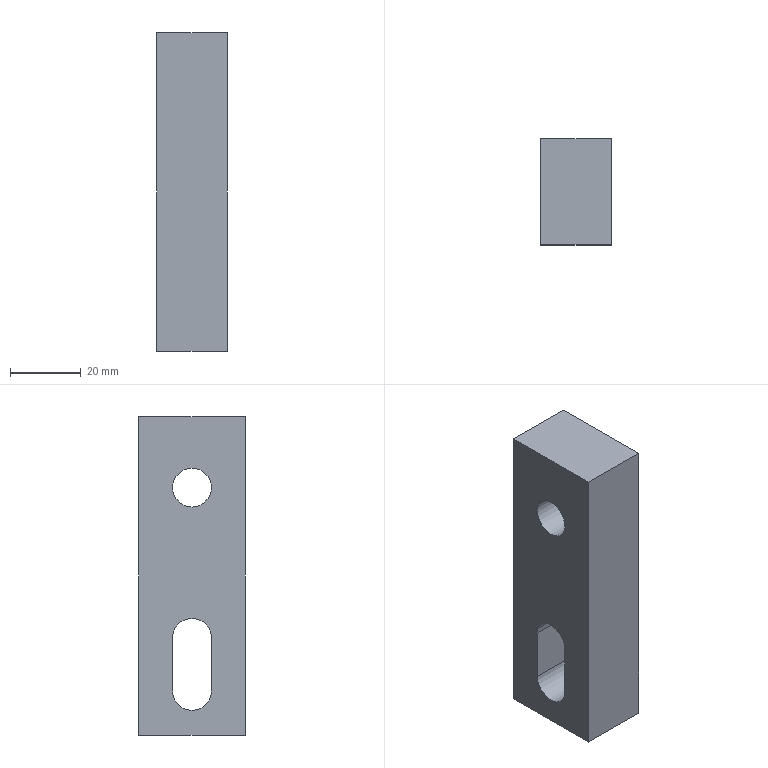Part | STEP file | solid 155 | 1 solid | 11 faces | box 20 x 30 x 90 mm | volume 46899 mm3 | plane 8 | cylinder 3 | commonest cylinder face diameters 11 x3